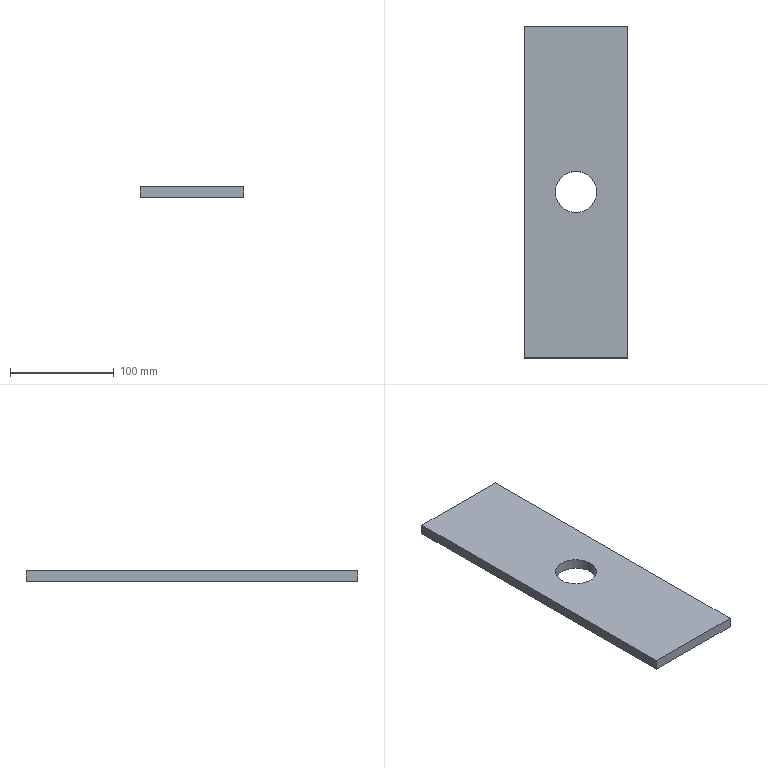Part | STEP file | A14-039 | 1 solid | 8 faces | box 100 x 320 x 10 mm | volume 307434 mm3 | plane 6 | cylinder 2 | commonest cylinder face diameters 40 x2
STEP:
#1=CARTESIAN_POINT('',(0.,0.,0.));
#2=DIRECTION('',(0.,0.,1.));
#3=DIRECTION('',(1.,0.,0.));
#4=AXIS2_PLACEMENT_3D('',#1,#2,#3);
#5=CARTESIAN_POINT('',(20.,0.,-5.));
#6=VERTEX_POINT('',#5);
#7=CARTESIAN_POINT('',(20.,0.,5.));
#8=VERTEX_POINT('',#7);
#9=CARTESIAN_POINT('',(20.,0.,-5.));
#10=DIRECTION('',(0.,0.,1.));
#11=VECTOR('',#10,1.);
#12=LINE('',#9,#11);
#13=CARTESIAN_POINT('',(0.,0.,-5.));
#14=DIRECTION('',(0.,0.,1.));
#15=DIRECTION('',(1.,0.,0.));
#16=AXIS2_PLACEMENT_3D('',#13,#14,#15);
#17=CYLINDRICAL_SURFACE('',#16,20.);
#18=CARTESIAN_POINT('',(6.283,0.));
#19=DIRECTION('',(0.,1.));
#20=VECTOR('',#19,1.);
#21=LINE('',#18,#20);
#22=(GEOMETRIC_REPRESENTATION_CONTEXT(2)PARAMETRIC_REPRESENTATION_CONTEXT()REPRESENTATION_CONTEXT('',''));
#23=DEFINITIONAL_REPRESENTATION('',(#21),#22);
#24=PCURVE('',#17,#23);
#25=CARTESIAN_POINT('',(0.,0.,-5.));
#26=DIRECTION('',(0.,0.,1.));
#27=DIRECTION('',(1.,0.,0.));
#28=AXIS2_PLACEMENT_3D('',#25,#26,#27);
#29=CYLINDRICAL_SURFACE('',#28,20.);
#30=CARTESIAN_POINT('',(0.,0.));
#31=DIRECTION('',(0.,1.));
#32=VECTOR('',#31,1.);
#33=LINE('',#30,#32);
#34=(GEOMETRIC_REPRESENTATION_CONTEXT(2)PARAMETRIC_REPRESENTATION_CONTEXT()REPRESENTATION_CONTEXT('',''));
#35=DEFINITIONAL_REPRESENTATION('',(#33),#34);
#36=PCURVE('',#29,#35);
#37=SURFACE_CURVE('',#12,(#24,#36),.PCURVE_S1.);
#38=EDGE_CURVE('',#6,#8,#37,.T.);
#39=ORIENTED_EDGE('',*,*,#38,.T.);
#40=CARTESIAN_POINT('',(-20.,0.,5.));
#41=VERTEX_POINT('',#40);
#42=CARTESIAN_POINT('',(0.,0.,5.));
#43=DIRECTION('',(0.,0.,1.));
#44=DIRECTION('',(1.,0.,0.));
#45=AXIS2_PLACEMENT_3D('',#42,#43,#44);
#46=CIRCLE('',#45,20.);
#47=CARTESIAN_POINT('',(0.,10.));
#48=DIRECTION('',(1.,0.));
#49=VECTOR('',#48,1.);
#50=LINE('',#47,#49);
#51=(GEOMETRIC_REPRESENTATION_CONTEXT(2)PARAMETRIC_REPRESENTATION_CONTEXT()REPRESENTATION_CONTEXT('',''));
#52=DEFINITIONAL_REPRESENTATION('',(#50),#51);
#53=PCURVE('',#17,#52);
#54=CARTESIAN_POINT('',(0.,0.,5.));
#55=DIRECTION('',(0.,0.,1.));
#56=DIRECTION('',(1.,0.,0.));
#57=AXIS2_PLACEMENT_3D('',#54,#55,#56);
#58=PLANE('',#57);
#59=CARTESIAN_POINT('',(0.,0.));
#60=DIRECTION('',(1.,0.));
#61=AXIS2_PLACEMENT_2D('',#59,#60);
#62=CIRCLE('',#61,20.);
#63=(GEOMETRIC_REPRESENTATION_CONTEXT(2)PARAMETRIC_REPRESENTATION_CONTEXT()REPRESENTATION_CONTEXT('',''));
#64=DEFINITIONAL_REPRESENTATION('',(#62),#63);
#65=PCURVE('',#58,#64);
#66=SURFACE_CURVE('',#46,(#53,#65),.PCURVE_S1.);
#67=EDGE_CURVE('',#41,#8,#66,.T.);
#68=ORIENTED_EDGE('',*,*,#67,.F.);
#69=CARTESIAN_POINT('',(-20.,0.,-5.));
#70=VERTEX_POINT('',#69);
#71=CARTESIAN_POINT('',(-20.,0.,-5.));
#72=DIRECTION('',(0.,0.,1.));
#73=VECTOR('',#72,1.);
#74=LINE('',#71,#73);
#75=CARTESIAN_POINT('',(3.142,0.));
#76=DIRECTION('',(0.,1.));
#77=VECTOR('',#76,1.);
#78=LINE('',#75,#77);
#79=(GEOMETRIC_REPRESENTATION_CONTEXT(2)PARAMETRIC_REPRESENTATION_CONTEXT()REPRESENTATION_CONTEXT('',''));
#80=DEFINITIONAL_REPRESENTATION('',(#78),#79);
#81=PCURVE('',#17,#80);
#82=CARTESIAN_POINT('',(3.142,0.));
#83=DIRECTION('',(0.,1.));
#84=VECTOR('',#83,1.);
#85=LINE('',#82,#84);
#86=(GEOMETRIC_REPRESENTATION_CONTEXT(2)PARAMETRIC_REPRESENTATION_CONTEXT()REPRESENTATION_CONTEXT('',''));
#87=DEFINITIONAL_REPRESENTATION('',(#85),#86);
#88=PCURVE('',#29,#87);
#89=SURFACE_CURVE('',#74,(#81,#88),.PCURVE_S1.);
#90=EDGE_CURVE('',#70,#41,#89,.T.);
#91=ORIENTED_EDGE('',*,*,#90,.F.);
#92=CARTESIAN_POINT('',(0.,0.,-5.));
#93=DIRECTION('',(0.,0.,1.));
#94=DIRECTION('',(1.,0.,0.));
#95=AXIS2_PLACEMENT_3D('',#92,#93,#94);
#96=CIRCLE('',#95,20.);
#97=CARTESIAN_POINT('',(0.,0.));
#98=DIRECTION('',(1.,0.));
#99=VECTOR('',#98,1.);
#100=LINE('',#97,#99);
#101=(GEOMETRIC_REPRESENTATION_CONTEXT(2)PARAMETRIC_REPRESENTATION_CONTEXT()REPRESENTATION_CONTEXT('',''));
#102=DEFINITIONAL_REPRESENTATION('',(#100),#101);
#103=PCURVE('',#17,#102);
#104=CARTESIAN_POINT('',(0.,0.,-5.));
#105=DIRECTION('',(0.,0.,1.));
#106=DIRECTION('',(1.,0.,0.));
#107=AXIS2_PLACEMENT_3D('',#104,#105,#106);
#108=PLANE('',#107);
#109=CARTESIAN_POINT('',(0.,0.));
#110=DIRECTION('',(1.,0.));
#111=AXIS2_PLACEMENT_2D('',#109,#110);
#112=CIRCLE('',#111,20.);
#113=(GEOMETRIC_REPRESENTATION_CONTEXT(2)PARAMETRIC_REPRESENTATION_CONTEXT()REPRESENTATION_CONTEXT('',''));
#114=DEFINITIONAL_REPRESENTATION('',(#112),#113);
#115=PCURVE('',#108,#114);
#116=SURFACE_CURVE('',#96,(#103,#115),.PCURVE_S1.);
#117=EDGE_CURVE('',#70,#6,#116,.T.);
#118=ORIENTED_EDGE('',*,*,#117,.T.);
#119=EDGE_LOOP('',(#39,#68,#91,#118));
#120=FACE_BOUND('',#119,.F.);
#121=ADVANCED_FACE('',(#120),#17,.F.);
#122=CARTESIAN_POINT('',(50.,-160.,-5.));
#123=VERTEX_POINT('',#122);
#124=CARTESIAN_POINT('',(50.,160.,-5.));
#125=VERTEX_POINT('',#124);
#126=CARTESIAN_POINT('',(50.,160.,-5.));
#127=DIRECTION('',(0.,1.,0.));
#128=VECTOR('',#127,1.);
#129=LINE('',#126,#128);
#130=CARTESIAN_POINT('',(50.,160.,5.));
#131=DIRECTION('',(-1.,0.,0.));
#132=DIRECTION('',(0.,0.,1.));
#133=AXIS2_PLACEMENT_3D('',#130,#131,#132);
#134=PLANE('',#133);
#135=CARTESIAN_POINT('',(-10.,0.));
#136=DIRECTION('',(0.,1.));
#137=VECTOR('',#136,1.);
#138=LINE('',#135,#137);
#139=(GEOMETRIC_REPRESENTATION_CONTEXT(2)PARAMETRIC_REPRESENTATION_CONTEXT()REPRESENTATION_CONTEXT('',''));
#140=DEFINITIONAL_REPRESENTATION('',(#138),#139);
#141=PCURVE('',#134,#140);
#142=CARTESIAN_POINT('',(50.,160.));
#143=DIRECTION('',(0.,1.));
#144=VECTOR('',#143,1.);
#145=LINE('',#142,#144);
#146=(GEOMETRIC_REPRESENTATION_CONTEXT(2)PARAMETRIC_REPRESENTATION_CONTEXT()REPRESENTATION_CONTEXT('',''));
#147=DEFINITIONAL_REPRESENTATION('',(#145),#146);
#148=PCURVE('',#108,#147);
#149=SURFACE_CURVE('',#129,(#141,#148),.PCURVE_S1.);
#150=EDGE_CURVE('',#123,#125,#149,.T.);
#151=ORIENTED_EDGE('',*,*,#150,.T.);
#152=CARTESIAN_POINT('',(50.,160.,5.));
#153=VERTEX_POINT('',#152);
#154=CARTESIAN_POINT('',(50.,160.,5.));
#155=DIRECTION('',(0.,0.,-1.));
#156=VECTOR('',#155,1.);
#157=LINE('',#154,#156);
#158=CARTESIAN_POINT('',(0.,0.));
#159=DIRECTION('',(-1.,0.));
#160=VECTOR('',#159,1.);
#161=LINE('',#158,#160);
#162=(GEOMETRIC_REPRESENTATION_CONTEXT(2)PARAMETRIC_REPRESENTATION_CONTEXT()REPRESENTATION_CONTEXT('',''));
#163=DEFINITIONAL_REPRESENTATION('',(#161),#162);
#164=PCURVE('',#134,#163);
#165=CARTESIAN_POINT('',(-50.,160.,5.));
#166=DIRECTION('',(0.,-1.,0.));
#167=DIRECTION('',(0.,0.,-1.));
#168=AXIS2_PLACEMENT_3D('',#165,#166,#167);
#169=PLANE('',#168);
#170=CARTESIAN_POINT('',(0.,100.));
#171=DIRECTION('',(1.,0.));
#172=VECTOR('',#171,1.);
#173=LINE('',#170,#172);
#174=(GEOMETRIC_REPRESENTATION_CONTEXT(2)PARAMETRIC_REPRESENTATION_CONTEXT()REPRESENTATION_CONTEXT('',''));
#175=DEFINITIONAL_REPRESENTATION('',(#173),#174);
#176=PCURVE('',#169,#175);
#177=SURFACE_CURVE('',#157,(#164,#176),.PCURVE_S1.);
#178=EDGE_CURVE('',#153,#125,#177,.T.);
#179=ORIENTED_EDGE('',*,*,#178,.F.);
#180=CARTESIAN_POINT('',(50.,-160.,5.));
#181=VERTEX_POINT('',#180);
#182=CARTESIAN_POINT('',(50.,160.,5.));
#183=DIRECTION('',(0.,1.,0.));
#184=VECTOR('',#183,1.);
#185=LINE('',#182,#184);
#186=CARTESIAN_POINT('',(0.,0.));
#187=DIRECTION('',(0.,1.));
#188=VECTOR('',#187,1.);
#189=LINE('',#186,#188);
#190=(GEOMETRIC_REPRESENTATION_CONTEXT(2)PARAMETRIC_REPRESENTATION_CONTEXT()REPRESENTATION_CONTEXT('',''));
#191=DEFINITIONAL_REPRESENTATION('',(#189),#190);
#192=PCURVE('',#134,#191);
#193=CARTESIAN_POINT('',(50.,160.));
#194=DIRECTION('',(0.,1.));
#195=VECTOR('',#194,1.);
#196=LINE('',#193,#195);
#197=(GEOMETRIC_REPRESENTATION_CONTEXT(2)PARAMETRIC_REPRESENTATION_CONTEXT()REPRESENTATION_CONTEXT('',''));
#198=DEFINITIONAL_REPRESENTATION('',(#196),#197);
#199=PCURVE('',#58,#198);
#200=SURFACE_CURVE('',#185,(#192,#199),.PCURVE_S1.);
#201=EDGE_CURVE('',#181,#153,#200,.T.);
#202=ORIENTED_EDGE('',*,*,#201,.F.);
#203=CARTESIAN_POINT('',(50.,-160.,5.));
#204=DIRECTION('',(0.,0.,-1.));
#205=VECTOR('',#204,1.);
#206=LINE('',#203,#205);
#207=CARTESIAN_POINT('',(0.,-320.));
#208=DIRECTION('',(-1.,0.));
#209=VECTOR('',#208,1.);
#210=LINE('',#207,#209);
#211=(GEOMETRIC_REPRESENTATION_CONTEXT(2)PARAMETRIC_REPRESENTATION_CONTEXT()REPRESENTATION_CONTEXT('',''));
#212=DEFINITIONAL_REPRESENTATION('',(#210),#211);
#213=PCURVE('',#134,#212);
#214=CARTESIAN_POINT('',(-50.,-160.,5.));
#215=DIRECTION('',(0.,1.,0.));
#216=DIRECTION('',(0.,0.,1.));
#217=AXIS2_PLACEMENT_3D('',#214,#215,#216);
#218=PLANE('',#217);
#219=CARTESIAN_POINT('',(0.,100.));
#220=DIRECTION('',(-1.,0.));
#221=VECTOR('',#220,1.);
#222=LINE('',#219,#221);
#223=(GEOMETRIC_REPRESENTATION_CONTEXT(2)PARAMETRIC_REPRESENTATION_CONTEXT()REPRESENTATION_CONTEXT('',''));
#224=DEFINITIONAL_REPRESENTATION('',(#222),#223);
#225=PCURVE('',#218,#224);
#226=SURFACE_CURVE('',#206,(#213,#225),.PCURVE_S1.);
#227=EDGE_CURVE('',#181,#123,#226,.T.);
#228=ORIENTED_EDGE('',*,*,#227,.T.);
#229=EDGE_LOOP('',(#151,#179,#202,#228));
#230=FACE_BOUND('',#229,.T.);
#231=ADVANCED_FACE('',(#230),#134,.F.);
#232=CARTESIAN_POINT('',(-50.,160.,-5.));
#233=VERTEX_POINT('',#232);
#234=CARTESIAN_POINT('',(-50.,160.,-5.));
#235=DIRECTION('',(-1.,0.,0.));
#236=VECTOR('',#235,1.);
#237=LINE('',#234,#236);
#238=CARTESIAN_POINT('',(10.,0.));
#239=DIRECTION('',(0.,-1.));
#240=VECTOR('',#239,1.);
#241=LINE('',#238,#240);
#242=(GEOMETRIC_REPRESENTATION_CONTEXT(2)PARAMETRIC_REPRESENTATION_CONTEXT()REPRESENTATION_CONTEXT('',''));
#243=DEFINITIONAL_REPRESENTATION('',(#241),#242);
#244=PCURVE('',#169,#243);
#245=CARTESIAN_POINT('',(-50.,160.));
#246=DIRECTION('',(-1.,0.));
#247=VECTOR('',#246,1.);
#248=LINE('',#245,#247);
#249=(GEOMETRIC_REPRESENTATION_CONTEXT(2)PARAMETRIC_REPRESENTATION_CONTEXT()REPRESENTATION_CONTEXT('',''));
#250=DEFINITIONAL_REPRESENTATION('',(#248),#249);
#251=PCURVE('',#108,#250);
#252=SURFACE_CURVE('',#237,(#244,#251),.PCURVE_S1.);
#253=EDGE_CURVE('',#125,#233,#252,.T.);
#254=ORIENTED_EDGE('',*,*,#253,.T.);
#255=CARTESIAN_POINT('',(-50.,160.,5.));
#256=VERTEX_POINT('',#255);
#257=CARTESIAN_POINT('',(-50.,160.,5.));
#258=DIRECTION('',(0.,0.,-1.));
#259=VECTOR('',#258,1.);
#260=LINE('',#257,#259);
#261=CARTESIAN_POINT('',(0.,0.));
#262=DIRECTION('',(1.,0.));
#263=VECTOR('',#262,1.);
#264=LINE('',#261,#263);
#265=(GEOMETRIC_REPRESENTATION_CONTEXT(2)PARAMETRIC_REPRESENTATION_CONTEXT()REPRESENTATION_CONTEXT('',''));
#266=DEFINITIONAL_REPRESENTATION('',(#264),#265);
#267=PCURVE('',#169,#266);
#268=CARTESIAN_POINT('',(-50.,160.,5.));
#269=DIRECTION('',(1.,0.,0.));
#270=DIRECTION('',(0.,0.,-1.));
#271=AXIS2_PLACEMENT_3D('',#268,#269,#270);
#272=PLANE('',#271);
#273=CARTESIAN_POINT('',(0.,0.));
#274=DIRECTION('',(1.,0.));
#275=VECTOR('',#274,1.);
#276=LINE('',#273,#275);
#277=(GEOMETRIC_REPRESENTATION_CONTEXT(2)PARAMETRIC_REPRESENTATION_CONTEXT()REPRESENTATION_CONTEXT('',''));
#278=DEFINITIONAL_REPRESENTATION('',(#276),#277);
#279=PCURVE('',#272,#278);
#280=SURFACE_CURVE('',#260,(#267,#279),.PCURVE_S1.);
#281=EDGE_CURVE('',#256,#233,#280,.T.);
#282=ORIENTED_EDGE('',*,*,#281,.F.);
#283=CARTESIAN_POINT('',(-50.,160.,5.));
#284=DIRECTION('',(-1.,0.,0.));
#285=VECTOR('',#284,1.);
#286=LINE('',#283,#285);
#287=CARTESIAN_POINT('',(0.,0.));
#288=DIRECTION('',(0.,-1.));
#289=VECTOR('',#288,1.);
#290=LINE('',#287,#289);
#291=(GEOMETRIC_REPRESENTATION_CONTEXT(2)PARAMETRIC_REPRESENTATION_CONTEXT()REPRESENTATION_CONTEXT('',''));
#292=DEFINITIONAL_REPRESENTATION('',(#290),#291);
#293=PCURVE('',#169,#292);
#294=CARTESIAN_POINT('',(-50.,160.));
#295=DIRECTION('',(-1.,0.));
#296=VECTOR('',#295,1.);
#297=LINE('',#294,#296);
#298=(GEOMETRIC_REPRESENTATION_CONTEXT(2)PARAMETRIC_REPRESENTATION_CONTEXT()REPRESENTATION_CONTEXT('',''));
#299=DEFINITIONAL_REPRESENTATION('',(#297),#298);
#300=PCURVE('',#58,#299);
#301=SURFACE_CURVE('',#286,(#293,#300),.PCURVE_S1.);
#302=EDGE_CURVE('',#153,#256,#301,.T.);
#303=ORIENTED_EDGE('',*,*,#302,.F.);
#304=ORIENTED_EDGE('',*,*,#178,.T.);
#305=EDGE_LOOP('',(#254,#282,#303,#304));
#306=FACE_BOUND('',#305,.T.);
#307=ADVANCED_FACE('',(#306),#169,.F.);
#308=CARTESIAN_POINT('',(-50.,-160.,-5.));
#309=VERTEX_POINT('',#308);
#310=CARTESIAN_POINT('',(-50.,160.,-5.));
#311=DIRECTION('',(0.,-1.,0.));
#312=VECTOR('',#311,1.);
#313=LINE('',#310,#312);
#314=CARTESIAN_POINT('',(10.,0.));
#315=DIRECTION('',(0.,-1.));
#316=VECTOR('',#315,1.);
#317=LINE('',#314,#316);
#318=(GEOMETRIC_REPRESENTATION_CONTEXT(2)PARAMETRIC_REPRESENTATION_CONTEXT()REPRESENTATION_CONTEXT('',''));
#319=DEFINITIONAL_REPRESENTATION('',(#317),#318);
#320=PCURVE('',#272,#319);
#321=CARTESIAN_POINT('',(-50.,160.));
#322=DIRECTION('',(0.,-1.));
#323=VECTOR('',#322,1.);
#324=LINE('',#321,#323);
#325=(GEOMETRIC_REPRESENTATION_CONTEXT(2)PARAMETRIC_REPRESENTATION_CONTEXT()REPRESENTATION_CONTEXT('',''));
#326=DEFINITIONAL_REPRESENTATION('',(#324),#325);
#327=PCURVE('',#108,#326);
#328=SURFACE_CURVE('',#313,(#320,#327),.PCURVE_S1.);
#329=EDGE_CURVE('',#233,#309,#328,.T.);
#330=ORIENTED_EDGE('',*,*,#329,.T.);
#331=CARTESIAN_POINT('',(-50.,-160.,5.));
#332=VERTEX_POINT('',#331);
#333=CARTESIAN_POINT('',(-50.,-160.,5.));
#334=DIRECTION('',(0.,0.,-1.));
#335=VECTOR('',#334,1.);
#336=LINE('',#333,#335);
#337=CARTESIAN_POINT('',(0.,-320.));
#338=DIRECTION('',(1.,0.));
#339=VECTOR('',#338,1.);
#340=LINE('',#337,#339);
#341=(GEOMETRIC_REPRESENTATION_CONTEXT(2)PARAMETRIC_REPRESENTATION_CONTEXT()REPRESENTATION_CONTEXT('',''));
#342=DEFINITIONAL_REPRESENTATION('',(#340),#341);
#343=PCURVE('',#272,#342);
#344=CARTESIAN_POINT('',(0.,0.));
#345=DIRECTION('',(-1.,0.));
#346=VECTOR('',#345,1.);
#347=LINE('',#344,#346);
#348=(GEOMETRIC_REPRESENTATION_CONTEXT(2)PARAMETRIC_REPRESENTATION_CONTEXT()REPRESENTATION_CONTEXT('',''));
#349=DEFINITIONAL_REPRESENTATION('',(#347),#348);
#350=PCURVE('',#218,#349);
#351=SURFACE_CURVE('',#336,(#343,#350),.PCURVE_S1.);
#352=EDGE_CURVE('',#332,#309,#351,.T.);
#353=ORIENTED_EDGE('',*,*,#352,.F.);
#354=CARTESIAN_POINT('',(-50.,160.,5.));
#355=DIRECTION('',(0.,-1.,0.));
#356=VECTOR('',#355,1.);
#357=LINE('',#354,#356);
#358=CARTESIAN_POINT('',(0.,0.));
#359=DIRECTION('',(0.,-1.));
#360=VECTOR('',#359,1.);
#361=LINE('',#358,#360);
#362=(GEOMETRIC_REPRESENTATION_CONTEXT(2)PARAMETRIC_REPRESENTATION_CONTEXT()REPRESENTATION_CONTEXT('',''));
#363=DEFINITIONAL_REPRESENTATION('',(#361),#362);
#364=PCURVE('',#272,#363);
#365=CARTESIAN_POINT('',(-50.,160.));
#366=DIRECTION('',(0.,-1.));
#367=VECTOR('',#366,1.);
#368=LINE('',#365,#367);
#369=(GEOMETRIC_REPRESENTATION_CONTEXT(2)PARAMETRIC_REPRESENTATION_CONTEXT()REPRESENTATION_CONTEXT('',''));
#370=DEFINITIONAL_REPRESENTATION('',(#368),#369);
#371=PCURVE('',#58,#370);
#372=SURFACE_CURVE('',#357,(#364,#371),.PCURVE_S1.);
#373=EDGE_CURVE('',#256,#332,#372,.T.);
#374=ORIENTED_EDGE('',*,*,#373,.F.);
#375=ORIENTED_EDGE('',*,*,#281,.T.);
#376=EDGE_LOOP('',(#330,#353,#374,#375));
#377=FACE_BOUND('',#376,.T.);
#378=ADVANCED_FACE('',(#377),#272,.F.);
#379=CARTESIAN_POINT('',(-50.,-160.,-5.));
#380=DIRECTION('',(1.,0.,0.));
#381=VECTOR('',#380,1.);
#382=LINE('',#379,#381);
#383=CARTESIAN_POINT('',(-10.,0.));
#384=DIRECTION('',(0.,1.));
#385=VECTOR('',#384,1.);
#386=LINE('',#383,#385);
#387=(GEOMETRIC_REPRESENTATION_CONTEXT(2)PARAMETRIC_REPRESENTATION_CONTEXT()REPRESENTATION_CONTEXT('',''));
#388=DEFINITIONAL_REPRESENTATION('',(#386),#387);
#389=PCURVE('',#218,#388);
#390=CARTESIAN_POINT('',(-50.,-160.));
#391=DIRECTION('',(1.,0.));
#392=VECTOR('',#391,1.);
#393=LINE('',#390,#392);
#394=(GEOMETRIC_REPRESENTATION_CONTEXT(2)PARAMETRIC_REPRESENTATION_CONTEXT()REPRESENTATION_CONTEXT('',''));
#395=DEFINITIONAL_REPRESENTATION('',(#393),#394);
#396=PCURVE('',#108,#395);
#397=SURFACE_CURVE('',#382,(#389,#396),.PCURVE_S1.);
#398=EDGE_CURVE('',#309,#123,#397,.T.);
#399=ORIENTED_EDGE('',*,*,#398,.T.);
#400=ORIENTED_EDGE('',*,*,#227,.F.);
#401=CARTESIAN_POINT('',(-50.,-160.,5.));
#402=DIRECTION('',(1.,0.,0.));
#403=VECTOR('',#402,1.);
#404=LINE('',#401,#403);
#405=CARTESIAN_POINT('',(0.,0.));
#406=DIRECTION('',(0.,1.));
#407=VECTOR('',#406,1.);
#408=LINE('',#405,#407);
#409=(GEOMETRIC_REPRESENTATION_CONTEXT(2)PARAMETRIC_REPRESENTATION_CONTEXT()REPRESENTATION_CONTEXT('',''));
#410=DEFINITIONAL_REPRESENTATION('',(#408),#409);
#411=PCURVE('',#218,#410);
#412=CARTESIAN_POINT('',(-50.,-160.));
#413=DIRECTION('',(1.,0.));
#414=VECTOR('',#413,1.);
#415=LINE('',#412,#414);
#416=(GEOMETRIC_REPRESENTATION_CONTEXT(2)PARAMETRIC_REPRESENTATION_CONTEXT()REPRESENTATION_CONTEXT('',''));
#417=DEFINITIONAL_REPRESENTATION('',(#415),#416);
#418=PCURVE('',#58,#417);
#419=SURFACE_CURVE('',#404,(#411,#418),.PCURVE_S1.);
#420=EDGE_CURVE('',#332,#181,#419,.T.);
#421=ORIENTED_EDGE('',*,*,#420,.F.);
#422=ORIENTED_EDGE('',*,*,#352,.T.);
#423=EDGE_LOOP('',(#399,#400,#421,#422));
#424=FACE_BOUND('',#423,.T.);
#425=ADVANCED_FACE('',(#424),#218,.F.);
#426=CARTESIAN_POINT('',(0.,0.,5.));
#427=DIRECTION('',(0.,0.,1.));
#428=DIRECTION('',(1.,0.,0.));
#429=AXIS2_PLACEMENT_3D('',#426,#427,#428);
#430=CIRCLE('',#429,20.);
#431=CARTESIAN_POINT('',(0.,0.));
#432=DIRECTION('',(1.,0.));
#433=AXIS2_PLACEMENT_2D('',#431,#432);
#434=CIRCLE('',#433,20.);
#435=(GEOMETRIC_REPRESENTATION_CONTEXT(2)PARAMETRIC_REPRESENTATION_CONTEXT()REPRESENTATION_CONTEXT('',''));
#436=DEFINITIONAL_REPRESENTATION('',(#434),#435);
#437=PCURVE('',#58,#436);
#438=CARTESIAN_POINT('',(0.,10.));
#439=DIRECTION('',(1.,0.));
#440=VECTOR('',#439,1.);
#441=LINE('',#438,#440);
#442=(GEOMETRIC_REPRESENTATION_CONTEXT(2)PARAMETRIC_REPRESENTATION_CONTEXT()REPRESENTATION_CONTEXT('',''));
#443=DEFINITIONAL_REPRESENTATION('',(#441),#442);
#444=PCURVE('',#29,#443);
#445=SURFACE_CURVE('',#430,(#437,#444),.PCURVE_S1.);
#446=EDGE_CURVE('',#8,#41,#445,.T.);
#447=ORIENTED_EDGE('',*,*,#446,.F.);
#448=ORIENTED_EDGE('',*,*,#67,.F.);
#449=EDGE_LOOP('',(#447,#448));
#450=FACE_BOUND('',#449,.T.);
#451=ORIENTED_EDGE('',*,*,#201,.T.);
#452=ORIENTED_EDGE('',*,*,#302,.T.);
#453=ORIENTED_EDGE('',*,*,#373,.T.);
#454=ORIENTED_EDGE('',*,*,#420,.T.);
#455=EDGE_LOOP('',(#451,#452,#453,#454));
#456=FACE_BOUND('',#455,.T.);
#457=ADVANCED_FACE('',(#450,#456),#58,.T.);
#458=CARTESIAN_POINT('',(0.,0.,-5.));
#459=DIRECTION('',(0.,0.,1.));
#460=DIRECTION('',(1.,0.,0.));
#461=AXIS2_PLACEMENT_3D('',#458,#459,#460);
#462=CIRCLE('',#461,20.);
#463=CARTESIAN_POINT('',(0.,0.));
#464=DIRECTION('',(1.,0.));
#465=AXIS2_PLACEMENT_2D('',#463,#464);
#466=CIRCLE('',#465,20.);
#467=(GEOMETRIC_REPRESENTATION_CONTEXT(2)PARAMETRIC_REPRESENTATION_CONTEXT()REPRESENTATION_CONTEXT('',''));
#468=DEFINITIONAL_REPRESENTATION('',(#466),#467);
#469=PCURVE('',#108,#468);
#470=CARTESIAN_POINT('',(0.,0.));
#471=DIRECTION('',(1.,0.));
#472=VECTOR('',#471,1.);
#473=LINE('',#470,#472);
#474=(GEOMETRIC_REPRESENTATION_CONTEXT(2)PARAMETRIC_REPRESENTATION_CONTEXT()REPRESENTATION_CONTEXT('',''));
#475=DEFINITIONAL_REPRESENTATION('',(#473),#474);
#476=PCURVE('',#29,#475);
#477=SURFACE_CURVE('',#462,(#469,#476),.PCURVE_S1.);
#478=EDGE_CURVE('',#6,#70,#477,.T.);
#479=ORIENTED_EDGE('',*,*,#478,.T.);
#480=ORIENTED_EDGE('',*,*,#117,.T.);
#481=EDGE_LOOP('',(#479,#480));
#482=FACE_BOUND('',#481,.T.);
#483=ORIENTED_EDGE('',*,*,#150,.F.);
#484=ORIENTED_EDGE('',*,*,#398,.F.);
#485=ORIENTED_EDGE('',*,*,#329,.F.);
#486=ORIENTED_EDGE('',*,*,#253,.F.);
#487=EDGE_LOOP('',(#483,#484,#485,#486));
#488=FACE_BOUND('',#487,.T.);
#489=ADVANCED_FACE('',(#482,#488),#108,.F.);
#490=ORIENTED_EDGE('',*,*,#446,.F.);
#491=ORIENTED_EDGE('',*,*,#38,.F.);
#492=ORIENTED_EDGE('',*,*,#478,.T.);
#493=ORIENTED_EDGE('',*,*,#90,.T.);
#494=EDGE_LOOP('',(#490,#491,#492,#493));
#495=FACE_BOUND('',#494,.F.);
#496=ADVANCED_FACE('',(#495),#29,.F.);
#497=CLOSED_SHELL('',(#121,#231,#307,#378,#425,#457,#489,#496));
#498=MANIFOLD_SOLID_BREP('',#497);
#499=(LENGTH_UNIT()NAMED_UNIT(*)SI_UNIT(.MILLI.,.METRE.));
#500=UNCERTAINTY_MEASURE_WITH_UNIT(LENGTH_MEASURE(0.0000001),#499,'','');
#501=(NAMED_UNIT(*)PLANE_ANGLE_UNIT()SI_UNIT($,.RADIAN.));
#502=(NAMED_UNIT(*)SI_UNIT($,.STERADIAN.)SOLID_ANGLE_UNIT());
#503=(GEOMETRIC_REPRESENTATION_CONTEXT(3)GLOBAL_UNCERTAINTY_ASSIGNED_CONTEXT((#500))GLOBAL_UNIT_ASSIGNED_CONTEXT((#499,#501,#502))REPRESENTATION_CONTEXT('',''));
#504=ADVANCED_BREP_SHAPE_REPRESENTATION('',(#4,#498),#503);